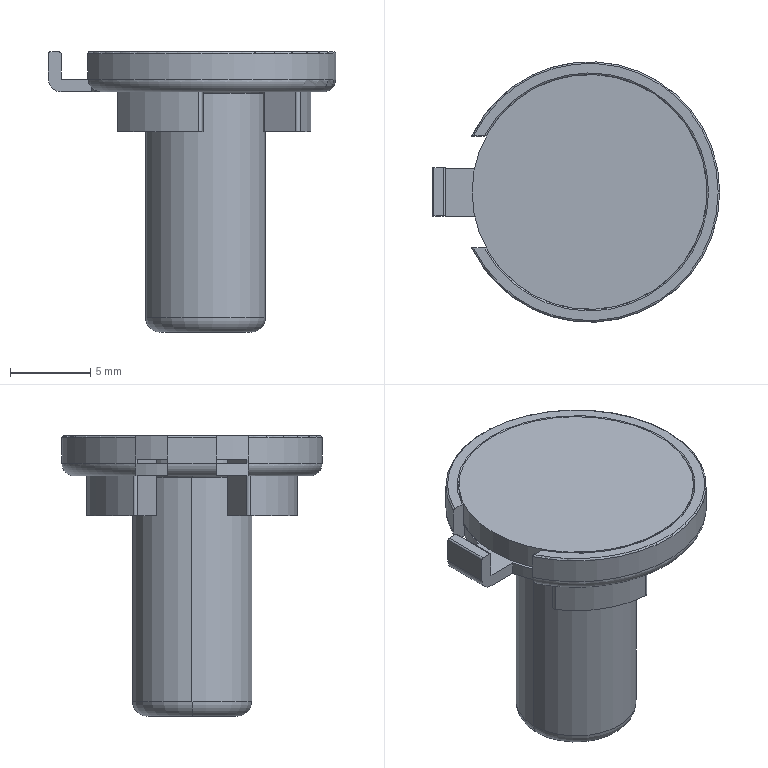Part | 2 solids | 108 faces | box 17.958 x 16.273 x 17.5 mm | volume 917.397 mm3 | cylinder 67 | plane 30 | torus 11 | commonest cylinder face diameters 0.4 x24 1 x16 8 x6 13.2 x6 5.9 x3 0.2 x2